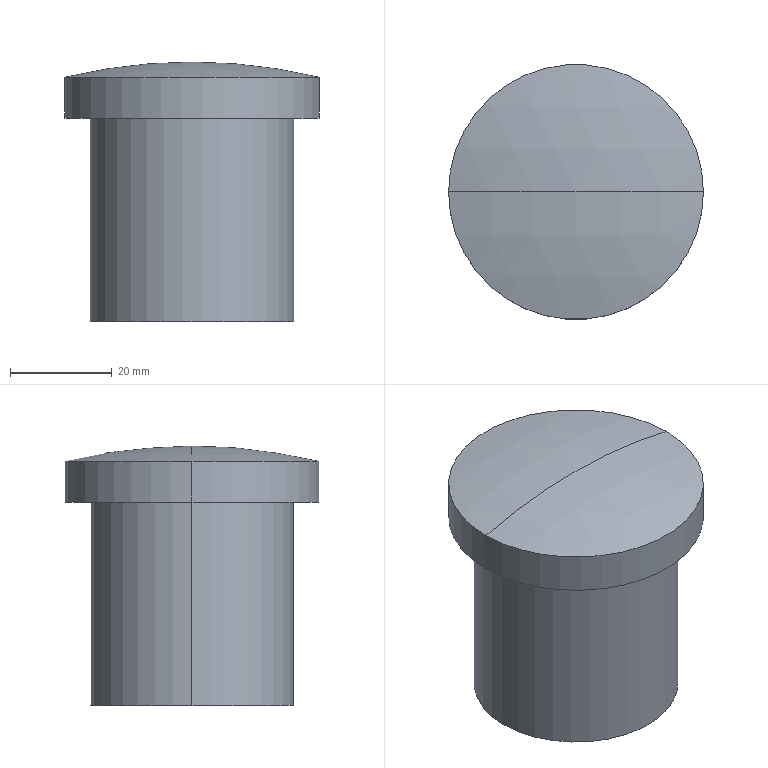Part | STEP file | Cylinder Joint | 1 solid | 11 faces | box 50 x 50 x 51 mm | volume 50075 mm3 | cylinder 6 | plane 3 | sphere 2 | commonest cylinder face diameters 24.5 x2 40 x2 50 x2
STEP:
#1=CARTESIAN_POINT('',(0.,0.,0.));
#2=DIRECTION('',(0.,0.,1.));
#3=DIRECTION('',(1.,0.,0.));
#4=AXIS2_PLACEMENT_3D('',#1,#2,#3);
#5=CARTESIAN_POINT('',(-12.25,0.,40.));
#6=VERTEX_POINT('',#5);
#7=CARTESIAN_POINT('',(-12.25,0.,0.));
#8=VERTEX_POINT('',#7);
#9=CARTESIAN_POINT('',(-12.25,0.,40.));
#10=DIRECTION('',(0.,0.,-1.));
#11=VECTOR('',#10,1.);
#12=LINE('',#9,#11);
#13=CARTESIAN_POINT('',(0.,0.,40.));
#14=DIRECTION('',(0.,0.,-1.));
#15=DIRECTION('',(-1.,0.,0.));
#16=AXIS2_PLACEMENT_3D('',#13,#14,#15);
#17=CYLINDRICAL_SURFACE('',#16,12.25);
#18=CARTESIAN_POINT('',(6.283,0.));
#19=DIRECTION('',(0.,1.));
#20=VECTOR('',#19,1.);
#21=LINE('',#18,#20);
#22=(GEOMETRIC_REPRESENTATION_CONTEXT(2)PARAMETRIC_REPRESENTATION_CONTEXT()REPRESENTATION_CONTEXT('',''));
#23=DEFINITIONAL_REPRESENTATION('',(#21),#22);
#24=PCURVE('',#17,#23);
#25=CARTESIAN_POINT('',(0.,0.,40.));
#26=DIRECTION('',(0.,0.,-1.));
#27=DIRECTION('',(-1.,0.,0.));
#28=AXIS2_PLACEMENT_3D('',#25,#26,#27);
#29=CYLINDRICAL_SURFACE('',#28,12.25);
#30=CARTESIAN_POINT('',(0.,0.));
#31=DIRECTION('',(0.,1.));
#32=VECTOR('',#31,1.);
#33=LINE('',#30,#32);
#34=(GEOMETRIC_REPRESENTATION_CONTEXT(2)PARAMETRIC_REPRESENTATION_CONTEXT()REPRESENTATION_CONTEXT('',''));
#35=DEFINITIONAL_REPRESENTATION('',(#33),#34);
#36=PCURVE('',#29,#35);
#37=SURFACE_CURVE('',#12,(#24,#36),.PCURVE_S1.);
#38=EDGE_CURVE('',#6,#8,#37,.T.);
#39=ORIENTED_EDGE('',*,*,#38,.T.);
#40=CARTESIAN_POINT('',(12.25,0.,0.));
#41=VERTEX_POINT('',#40);
#42=CARTESIAN_POINT('',(0.,0.,0.));
#43=DIRECTION('',(0.,0.,-1.));
#44=DIRECTION('',(-1.,0.,0.));
#45=AXIS2_PLACEMENT_3D('',#42,#43,#44);
#46=CIRCLE('',#45,12.25);
#47=CARTESIAN_POINT('',(0.,40.));
#48=DIRECTION('',(1.,0.));
#49=VECTOR('',#48,1.);
#50=LINE('',#47,#49);
#51=(GEOMETRIC_REPRESENTATION_CONTEXT(2)PARAMETRIC_REPRESENTATION_CONTEXT()REPRESENTATION_CONTEXT('',''));
#52=DEFINITIONAL_REPRESENTATION('',(#50),#51);
#53=PCURVE('',#17,#52);
#54=CARTESIAN_POINT('',(0.,0.,0.));
#55=DIRECTION('',(0.,0.,1.));
#56=DIRECTION('',(1.,0.,0.));
#57=AXIS2_PLACEMENT_3D('',#54,#55,#56);
#58=PLANE('',#57);
#59=CARTESIAN_POINT('',(-12.25,0.));
#60=CARTESIAN_POINT('',(-12.25,21.218));
#61=CARTESIAN_POINT('',(6.125,10.609));
#62=CARTESIAN_POINT('',(24.5,0.));
#63=CARTESIAN_POINT('',(6.125,-10.609));
#64=CARTESIAN_POINT('',(-12.25,-21.218));
#65=CARTESIAN_POINT('',(-12.25,0.));
#66=(BOUNDED_CURVE()B_SPLINE_CURVE(2,(#59,#60,#61,#62,#63,#64,#65),.UNSPECIFIED.,.T.,.F.)B_SPLINE_CURVE_WITH_KNOTS((1,2,2,2,2,1),(-2.094,0.,2.094,4.189,6.283,8.378),.UNSPECIFIED.)CURVE()GEOMETRIC_REPRESENTATION_ITEM()RATIONAL_B_SPLINE_CURVE((1.,0.5,1.,0.5,1.,0.5,1.))REPRESENTATION_ITEM(''));
#67=(GEOMETRIC_REPRESENTATION_CONTEXT(2)PARAMETRIC_REPRESENTATION_CONTEXT()REPRESENTATION_CONTEXT('',''));
#68=DEFINITIONAL_REPRESENTATION('',(#66),#67);
#69=PCURVE('',#58,#68);
#70=SURFACE_CURVE('',#46,(#53,#69),.PCURVE_S1.);
#71=EDGE_CURVE('',#41,#8,#70,.T.);
#72=ORIENTED_EDGE('',*,*,#71,.F.);
#73=CARTESIAN_POINT('',(12.25,0.,40.));
#74=VERTEX_POINT('',#73);
#75=CARTESIAN_POINT('',(12.25,0.,40.));
#76=DIRECTION('',(0.,0.,-1.));
#77=VECTOR('',#76,1.);
#78=LINE('',#75,#77);
#79=CARTESIAN_POINT('',(3.142,0.));
#80=DIRECTION('',(0.,1.));
#81=VECTOR('',#80,1.);
#82=LINE('',#79,#81);
#83=(GEOMETRIC_REPRESENTATION_CONTEXT(2)PARAMETRIC_REPRESENTATION_CONTEXT()REPRESENTATION_CONTEXT('',''));
#84=DEFINITIONAL_REPRESENTATION('',(#82),#83);
#85=PCURVE('',#17,#84);
#86=CARTESIAN_POINT('',(3.142,0.));
#87=DIRECTION('',(0.,1.));
#88=VECTOR('',#87,1.);
#89=LINE('',#86,#88);
#90=(GEOMETRIC_REPRESENTATION_CONTEXT(2)PARAMETRIC_REPRESENTATION_CONTEXT()REPRESENTATION_CONTEXT('',''));
#91=DEFINITIONAL_REPRESENTATION('',(#89),#90);
#92=PCURVE('',#29,#91);
#93=SURFACE_CURVE('',#78,(#85,#92),.PCURVE_S1.);
#94=EDGE_CURVE('',#74,#41,#93,.T.);
#95=ORIENTED_EDGE('',*,*,#94,.F.);
#96=CARTESIAN_POINT('',(0.,0.,40.));
#97=DIRECTION('',(0.,0.,-1.));
#98=DIRECTION('',(-1.,0.,0.));
#99=AXIS2_PLACEMENT_3D('',#96,#97,#98);
#100=CIRCLE('',#99,12.25);
#101=CARTESIAN_POINT('',(0.,0.));
#102=DIRECTION('',(1.,0.));
#103=VECTOR('',#102,1.);
#104=LINE('',#101,#103);
#105=(GEOMETRIC_REPRESENTATION_CONTEXT(2)PARAMETRIC_REPRESENTATION_CONTEXT()REPRESENTATION_CONTEXT('',''));
#106=DEFINITIONAL_REPRESENTATION('',(#104),#105);
#107=PCURVE('',#17,#106);
#108=CARTESIAN_POINT('',(0.,0.,40.));
#109=DIRECTION('',(0.,0.,-1.));
#110=DIRECTION('',(-1.,0.,0.));
#111=AXIS2_PLACEMENT_3D('',#108,#109,#110);
#112=PLANE('',#111);
#113=CARTESIAN_POINT('',(0.,0.));
#114=DIRECTION('',(1.,0.));
#115=AXIS2_PLACEMENT_2D('',#113,#114);
#116=CIRCLE('',#115,12.25);
#117=(GEOMETRIC_REPRESENTATION_CONTEXT(2)PARAMETRIC_REPRESENTATION_CONTEXT()REPRESENTATION_CONTEXT('',''));
#118=DEFINITIONAL_REPRESENTATION('',(#116),#117);
#119=PCURVE('',#112,#118);
#120=SURFACE_CURVE('',#100,(#107,#119),.PCURVE_S1.);
#121=EDGE_CURVE('',#74,#6,#120,.T.);
#122=ORIENTED_EDGE('',*,*,#121,.T.);
#123=EDGE_LOOP('',(#39,#72,#95,#122));
#124=FACE_BOUND('',#123,.F.);
#125=ADVANCED_FACE('',(#124),#17,.F.);
#126=CARTESIAN_POINT('',(25.,0.,48.));
#127=VERTEX_POINT('',#126);
#128=CARTESIAN_POINT('',(-25.,0.,48.));
#129=VERTEX_POINT('',#128);
#130=CARTESIAN_POINT('',(0.,0.,48.));
#131=DIRECTION('',(0.,0.,1.));
#132=DIRECTION('',(1.,0.,0.));
#133=AXIS2_PLACEMENT_3D('',#130,#131,#132);
#134=CIRCLE('',#133,25.);
#135=CARTESIAN_POINT('',(0.,0.,-54.667));
#136=DIRECTION('',(0.,1.,0.));
#137=DIRECTION('',(1.,0.,0.));
#138=AXIS2_PLACEMENT_3D('',#135,#136,#137);
#139=SPHERICAL_SURFACE('',#138,105.667);
#140=CARTESIAN_POINT('',(4.951,0.));
#141=CARTESIAN_POINT('',(4.951,0.01126));
#142=CARTESIAN_POINT('',(4.95,0.03379));
#143=CARTESIAN_POINT('',(4.943,0.06692));
#144=CARTESIAN_POINT('',(4.931,0.09876));
#145=CARTESIAN_POINT('',(4.915,0.1287));
#146=CARTESIAN_POINT('',(4.895,0.1561));
#147=CARTESIAN_POINT('',(4.871,0.1804));
#148=CARTESIAN_POINT('',(4.844,0.2011));
#149=CARTESIAN_POINT('',(4.814,0.2177));
#150=CARTESIAN_POINT('',(4.781,0.2298));
#151=CARTESIAN_POINT('',(4.747,0.2372));
#152=CARTESIAN_POINT('',(4.712,0.2397));
#153=CARTESIAN_POINT('',(4.678,0.2372));
#154=CARTESIAN_POINT('',(4.644,0.2298));
#155=CARTESIAN_POINT('',(4.611,0.2177));
#156=CARTESIAN_POINT('',(4.581,0.2011));
#157=CARTESIAN_POINT('',(4.554,0.1804));
#158=CARTESIAN_POINT('',(4.53,0.1561));
#159=CARTESIAN_POINT('',(4.51,0.1287));
#160=CARTESIAN_POINT('',(4.494,0.09876));
#161=CARTESIAN_POINT('',(4.482,0.06692));
#162=CARTESIAN_POINT('',(4.475,0.03379));
#163=CARTESIAN_POINT('',(4.474,0.01126));
#164=CARTESIAN_POINT('',(4.474,0.));
#165=B_SPLINE_CURVE_WITH_KNOTS('',3,(#140,#141,#142,#143,#144,#145,#146,#147,#148,#149,#150,#151,#152,#153,#154,#155,#156,#157,#158,#159,#160,#161,#162,#163,#164),.UNSPECIFIED.,.F.,.F.,(4,1,1,1,1,1,1,1,1,1,1,1,1,1,1,1,1,1,1,1,1,1,4),(0.,0.1428,0.2856,0.4284,0.5712,0.714,0.8568,0.9996,1.142,1.285,1.428,1.571,1.714,1.856,1.999,2.142,2.285,2.428,2.57,2.713,2.856,2.999,3.142),.QUASI_UNIFORM_KNOTS.);
#166=(GEOMETRIC_REPRESENTATION_CONTEXT(2)PARAMETRIC_REPRESENTATION_CONTEXT()REPRESENTATION_CONTEXT('',''));
#167=DEFINITIONAL_REPRESENTATION('',(#165),#166);
#168=PCURVE('',#139,#167);
#169=CARTESIAN_POINT('',(0.,0.,48.));
#170=DIRECTION('',(0.,0.,-1.));
#171=DIRECTION('',(-1.,0.,0.));
#172=AXIS2_PLACEMENT_3D('',#169,#170,#171);
#173=CYLINDRICAL_SURFACE('',#172,25.);
#174=CARTESIAN_POINT('',(3.142,0.));
#175=DIRECTION('',(-1.,0.));
#176=VECTOR('',#175,1.);
#177=LINE('',#174,#176);
#178=(GEOMETRIC_REPRESENTATION_CONTEXT(2)PARAMETRIC_REPRESENTATION_CONTEXT()REPRESENTATION_CONTEXT('',''));
#179=DEFINITIONAL_REPRESENTATION('',(#177),#178);
#180=PCURVE('',#173,#179);
#181=SURFACE_CURVE('',#134,(#168,#180),.PCURVE_S1.);
#182=EDGE_CURVE('',#127,#129,#181,.T.);
#183=ORIENTED_EDGE('',*,*,#182,.T.);
#184=CARTESIAN_POINT('',(0.,0.,51.));
#185=VERTEX_POINT('',#184);
#186=CARTESIAN_POINT('',(0.,0.,-54.667));
#187=DIRECTION('',(0.,1.,0.));
#188=DIRECTION('',(-1.,0.,0.));
#189=AXIS2_PLACEMENT_3D('',#186,#187,#188);
#190=CIRCLE('',#189,105.667);
#191=CARTESIAN_POINT('',(3.142,0.));
#192=DIRECTION('',(1.,0.));
#193=VECTOR('',#192,1.);
#194=LINE('',#191,#193);
#195=(GEOMETRIC_REPRESENTATION_CONTEXT(2)PARAMETRIC_REPRESENTATION_CONTEXT()REPRESENTATION_CONTEXT('',''));
#196=DEFINITIONAL_REPRESENTATION('',(#194),#195);
#197=PCURVE('',#139,#196);
#198=CARTESIAN_POINT('',(0.,0.,-54.667));
#199=DIRECTION('',(0.,1.,0.));
#200=DIRECTION('',(1.,0.,0.));
#201=AXIS2_PLACEMENT_3D('',#198,#199,#200);
#202=SPHERICAL_SURFACE('',#201,105.667);
#203=CARTESIAN_POINT('',(3.142,0.));
#204=DIRECTION('',(1.,0.));
#205=VECTOR('',#204,1.);
#206=LINE('',#203,#205);
#207=(GEOMETRIC_REPRESENTATION_CONTEXT(2)PARAMETRIC_REPRESENTATION_CONTEXT()REPRESENTATION_CONTEXT('',''));
#208=DEFINITIONAL_REPRESENTATION('',(#206),#207);
#209=PCURVE('',#202,#208);
#210=SURFACE_CURVE('',#190,(#197,#209),.PCURVE_S1.);
#211=EDGE_CURVE('',#129,#185,#210,.T.);
#212=ORIENTED_EDGE('',*,*,#211,.T.);
#213=CARTESIAN_POINT('',(0.,0.,-54.667));
#214=DIRECTION('',(0.,-1.,0.));
#215=DIRECTION('',(0.,0.,-1.));
#216=AXIS2_PLACEMENT_3D('',#213,#214,#215);
#217=CIRCLE('',#216,105.667);
#218=CARTESIAN_POINT('',(7.854,0.));
#219=DIRECTION('',(-1.,0.));
#220=VECTOR('',#219,1.);
#221=LINE('',#218,#220);
#222=(GEOMETRIC_REPRESENTATION_CONTEXT(2)PARAMETRIC_REPRESENTATION_CONTEXT()REPRESENTATION_CONTEXT('',''));
#223=DEFINITIONAL_REPRESENTATION('',(#221),#222);
#224=PCURVE('',#139,#223);
#225=CARTESIAN_POINT('',(7.854,0.));
#226=DIRECTION('',(-1.,0.));
#227=VECTOR('',#226,1.);
#228=LINE('',#225,#227);
#229=(GEOMETRIC_REPRESENTATION_CONTEXT(2)PARAMETRIC_REPRESENTATION_CONTEXT()REPRESENTATION_CONTEXT('',''));
#230=DEFINITIONAL_REPRESENTATION('',(#228),#229);
#231=PCURVE('',#202,#230);
#232=SURFACE_CURVE('',#217,(#224,#231),.PCURVE_S1.);
#233=EDGE_CURVE('',#127,#185,#232,.T.);
#234=ORIENTED_EDGE('',*,*,#233,.F.);
#235=EDGE_LOOP('',(#183,#212,#234));
#236=FACE_BOUND('',#235,.T.);
#237=ADVANCED_FACE('',(#236),#139,.T.);
#238=ORIENTED_EDGE('',*,*,#182,.F.);
#239=CARTESIAN_POINT('',(25.,0.,40.));
#240=VERTEX_POINT('',#239);
#241=CARTESIAN_POINT('',(25.,0.,48.));
#242=DIRECTION('',(0.,0.,-1.));
#243=VECTOR('',#242,1.);
#244=LINE('',#241,#243);
#245=CARTESIAN_POINT('',(3.142,0.));
#246=DIRECTION('',(0.,1.));
#247=VECTOR('',#246,1.);
#248=LINE('',#245,#247);
#249=(GEOMETRIC_REPRESENTATION_CONTEXT(2)PARAMETRIC_REPRESENTATION_CONTEXT()REPRESENTATION_CONTEXT('',''));
#250=DEFINITIONAL_REPRESENTATION('',(#248),#249);
#251=PCURVE('',#173,#250);
#252=CARTESIAN_POINT('',(0.,0.,48.));
#253=DIRECTION('',(0.,0.,-1.));
#254=DIRECTION('',(-1.,0.,0.));
#255=AXIS2_PLACEMENT_3D('',#252,#253,#254);
#256=CYLINDRICAL_SURFACE('',#255,25.);
#257=CARTESIAN_POINT('',(3.142,0.));
#258=DIRECTION('',(0.,1.));
#259=VECTOR('',#258,1.);
#260=LINE('',#257,#259);
#261=(GEOMETRIC_REPRESENTATION_CONTEXT(2)PARAMETRIC_REPRESENTATION_CONTEXT()REPRESENTATION_CONTEXT('',''));
#262=DEFINITIONAL_REPRESENTATION('',(#260),#261);
#263=PCURVE('',#256,#262);
#264=SURFACE_CURVE('',#244,(#251,#263),.PCURVE_S1.);
#265=EDGE_CURVE('',#127,#240,#264,.T.);
#266=ORIENTED_EDGE('',*,*,#265,.T.);
#267=CARTESIAN_POINT('',(-25.,0.,40.));
#268=VERTEX_POINT('',#267);
#269=CARTESIAN_POINT('',(0.,0.,40.));
#270=DIRECTION('',(0.,0.,1.));
#271=DIRECTION('',(1.,0.,0.));
#272=AXIS2_PLACEMENT_3D('',#269,#270,#271);
#273=CIRCLE('',#272,25.);
#274=CARTESIAN_POINT('',(3.142,8.));
#275=DIRECTION('',(-1.,0.));
#276=VECTOR('',#275,1.);
#277=LINE('',#274,#276);
#278=(GEOMETRIC_REPRESENTATION_CONTEXT(2)PARAMETRIC_REPRESENTATION_CONTEXT()REPRESENTATION_CONTEXT('',''));
#279=DEFINITIONAL_REPRESENTATION('',(#277),#278);
#280=PCURVE('',#173,#279);
#281=CARTESIAN_POINT('',(0.,0.,40.));
#282=DIRECTION('',(0.,0.,1.));
#283=DIRECTION('',(1.,0.,0.));
#284=AXIS2_PLACEMENT_3D('',#281,#282,#283);
#285=PLANE('',#284);
#286=CARTESIAN_POINT('',(0.,0.));
#287=DIRECTION('',(1.,0.));
#288=AXIS2_PLACEMENT_2D('',#286,#287);
#289=CIRCLE('',#288,25.);
#290=(GEOMETRIC_REPRESENTATION_CONTEXT(2)PARAMETRIC_REPRESENTATION_CONTEXT()REPRESENTATION_CONTEXT('',''));
#291=DEFINITIONAL_REPRESENTATION('',(#289),#290);
#292=PCURVE('',#285,#291);
#293=SURFACE_CURVE('',#273,(#280,#292),.PCURVE_S1.);
#294=EDGE_CURVE('',#240,#268,#293,.T.);
#295=ORIENTED_EDGE('',*,*,#294,.T.);
#296=CARTESIAN_POINT('',(-25.,0.,48.));
#297=DIRECTION('',(0.,0.,-1.));
#298=VECTOR('',#297,1.);
#299=LINE('',#296,#298);
#300=CARTESIAN_POINT('',(0.,0.));
#301=DIRECTION('',(0.,1.));
#302=VECTOR('',#301,1.);
#303=LINE('',#300,#302);
#304=(GEOMETRIC_REPRESENTATION_CONTEXT(2)PARAMETRIC_REPRESENTATION_CONTEXT()REPRESENTATION_CONTEXT('',''));
#305=DEFINITIONAL_REPRESENTATION('',(#303),#304);
#306=PCURVE('',#173,#305);
#307=CARTESIAN_POINT('',(6.283,0.));
#308=DIRECTION('',(0.,1.));
#309=VECTOR('',#308,1.);
#310=LINE('',#307,#309);
#311=(GEOMETRIC_REPRESENTATION_CONTEXT(2)PARAMETRIC_REPRESENTATION_CONTEXT()REPRESENTATION_CONTEXT('',''));
#312=DEFINITIONAL_REPRESENTATION('',(#310),#311);
#313=PCURVE('',#256,#312);
#314=SURFACE_CURVE('',#299,(#306,#313),.PCURVE_S1.);
#315=EDGE_CURVE('',#129,#268,#314,.T.);
#316=ORIENTED_EDGE('',*,*,#315,.F.);
#317=EDGE_LOOP('',(#238,#266,#295,#316));
#318=FACE_BOUND('',#317,.T.);
#319=ADVANCED_FACE('',(#318),#173,.T.);
#320=CARTESIAN_POINT('',(20.,0.,40.));
#321=VERTEX_POINT('',#320);
#322=CARTESIAN_POINT('',(-20.,0.,40.));
#323=VERTEX_POINT('',#322);
#324=CARTESIAN_POINT('',(0.,0.,40.));
#325=DIRECTION('',(0.,0.,1.));
#326=DIRECTION('',(1.,0.,0.));
#327=AXIS2_PLACEMENT_3D('',#324,#325,#326);
#328=CIRCLE('',#327,20.);
#329=CARTESIAN_POINT('',(0.,0.,40.));
#330=DIRECTION('',(0.,0.,-1.));
#331=DIRECTION('',(-1.,0.,0.));
#332=AXIS2_PLACEMENT_3D('',#329,#330,#331);
#333=CYLINDRICAL_SURFACE('',#332,20.);
#334=CARTESIAN_POINT('',(3.142,0.));
#335=DIRECTION('',(-1.,0.));
#336=VECTOR('',#335,1.);
#337=LINE('',#334,#336);
#338=(GEOMETRIC_REPRESENTATION_CONTEXT(2)PARAMETRIC_REPRESENTATION_CONTEXT()REPRESENTATION_CONTEXT('',''));
#339=DEFINITIONAL_REPRESENTATION('',(#337),#338);
#340=PCURVE('',#333,#339);
#341=CARTESIAN_POINT('',(0.,0.));
#342=DIRECTION('',(1.,0.));
#343=AXIS2_PLACEMENT_2D('',#341,#342);
#344=CIRCLE('',#343,20.);
#345=(GEOMETRIC_REPRESENTATION_CONTEXT(2)PARAMETRIC_REPRESENTATION_CONTEXT()REPRESENTATION_CONTEXT('',''));
#346=DEFINITIONAL_REPRESENTATION('',(#344),#345);
#347=PCURVE('',#285,#346);
#348=SURFACE_CURVE('',#328,(#340,#347),.PCURVE_S1.);
#349=EDGE_CURVE('',#321,#323,#348,.T.);
#350=ORIENTED_EDGE('',*,*,#349,.F.);
#351=CARTESIAN_POINT('',(20.,0.,0.));
#352=VERTEX_POINT('',#351);
#353=CARTESIAN_POINT('',(20.,0.,40.));
#354=DIRECTION('',(0.,0.,-1.));
#355=VECTOR('',#354,1.);
#356=LINE('',#353,#355);
#357=CARTESIAN_POINT('',(3.142,0.));
#358=DIRECTION('',(0.,1.));
#359=VECTOR('',#358,1.);
#360=LINE('',#357,#359);
#361=(GEOMETRIC_REPRESENTATION_CONTEXT(2)PARAMETRIC_REPRESENTATION_CONTEXT()REPRESENTATION_CONTEXT('',''));
#362=DEFINITIONAL_REPRESENTATION('',(#360),#361);
#363=PCURVE('',#333,#362);
#364=CARTESIAN_POINT('',(0.,0.,40.));
#365=DIRECTION('',(0.,0.,-1.));
#366=DIRECTION('',(-1.,0.,0.));
#367=AXIS2_PLACEMENT_3D('',#364,#365,#366);
#368=CYLINDRICAL_SURFACE('',#367,20.);
#369=CARTESIAN_POINT('',(3.142,0.));
#370=DIRECTION('',(0.,1.));
#371=VECTOR('',#370,1.);
#372=LINE('',#369,#371);
#373=(GEOMETRIC_REPRESENTATION_CONTEXT(2)PARAMETRIC_REPRESENTATION_CONTEXT()REPRESENTATION_CONTEXT('',''));
#374=DEFINITIONAL_REPRESENTATION('',(#372),#373);
#375=PCURVE('',#368,#374);
#376=SURFACE_CURVE('',#356,(#363,#375),.PCURVE_S1.);
#377=EDGE_CURVE('',#321,#352,#376,.T.);
#378=ORIENTED_EDGE('',*,*,#377,.T.);
#379=CARTESIAN_POINT('',(-20.,0.,0.));
#380=VERTEX_POINT('',#379);
#381=CARTESIAN_POINT('',(0.,0.,0.));
#382=DIRECTION('',(0.,0.,1.));
#383=DIRECTION('',(1.,0.,0.));
#384=AXIS2_PLACEMENT_3D('',#381,#382,#383);
#385=CIRCLE('',#384,20.);
#386=CARTESIAN_POINT('',(3.142,40.));
#387=DIRECTION('',(-1.,0.));
#388=VECTOR('',#387,1.);
#389=LINE('',#386,#388);
#390=(GEOMETRIC_REPRESENTATION_CONTEXT(2)PARAMETRIC_REPRESENTATION_CONTEXT()REPRESENTATION_CONTEXT('',''));
#391=DEFINITIONAL_REPRESENTATION('',(#389),#390);
#392=PCURVE('',#333,#391);
#393=CARTESIAN_POINT('',(0.,0.));
#394=DIRECTION('',(1.,0.));
#395=AXIS2_PLACEMENT_2D('',#393,#394);
#396=CIRCLE('',#395,20.);
#397=(GEOMETRIC_REPRESENTATION_CONTEXT(2)PARAMETRIC_REPRESENTATION_CONTEXT()REPRESENTATION_CONTEXT('',''));
#398=DEFINITIONAL_REPRESENTATION('',(#396),#397);
#399=PCURVE('',#58,#398);
#400=SURFACE_CURVE('',#385,(#392,#399),.PCURVE_S1.);
#401=EDGE_CURVE('',#352,#380,#400,.T.);
#402=ORIENTED_EDGE('',*,*,#401,.T.);
#403=CARTESIAN_POINT('',(-20.,0.,40.));
#404=DIRECTION('',(0.,0.,-1.));
#405=VECTOR('',#404,1.);
#406=LINE('',#403,#405);
#407=CARTESIAN_POINT('',(0.,0.));
#408=DIRECTION('',(0.,1.));
#409=VECTOR('',#408,1.);
#410=LINE('',#407,#409);
#411=(GEOMETRIC_REPRESENTATION_CONTEXT(2)PARAMETRIC_REPRESENTATION_CONTEXT()REPRESENTATION_CONTEXT('',''));
#412=DEFINITIONAL_REPRESENTATION('',(#410),#411);
#413=PCURVE('',#333,#412);
#414=CARTESIAN_POINT('',(6.283,0.));
#415=DIRECTION('',(0.,1.));
#416=VECTOR('',#415,1.);
#417=LINE('',#414,#416);
#418=(GEOMETRIC_REPRESENTATION_CONTEXT(2)PARAMETRIC_REPRESENTATION_CONTEXT()REPRESENTATION_CONTEXT('',''));
#419=DEFINITIONAL_REPRESENTATION('',(#417),#418);
#420=PCURVE('',#368,#419);
#421=SURFACE_CURVE('',#406,(#413,#420),.PCURVE_S1.);
#422=EDGE_CURVE('',#323,#380,#421,.T.);
#423=ORIENTED_EDGE('',*,*,#422,.F.);
#424=EDGE_LOOP('',(#350,#378,#402,#423));
#425=FACE_BOUND('',#424,.T.);
#426=ADVANCED_FACE('',(#425),#333,.T.);
#427=ORIENTED_EDGE('',*,*,#377,.F.);
#428=CARTESIAN_POINT('',(0.,0.,40.));
#429=DIRECTION('',(0.,0.,1.));
#430=DIRECTION('',(1.,0.,0.));
#431=AXIS2_PLACEMENT_3D('',#428,#429,#430);
#432=CIRCLE('',#431,20.);
#433=CARTESIAN_POINT('',(9.425,0.));
#434=DIRECTION('',(-1.,0.));
#435=VECTOR('',#434,1.);
#436=LINE('',#433,#435);
#437=(GEOMETRIC_REPRESENTATION_CONTEXT(2)PARAMETRIC_REPRESENTATION_CONTEXT()REPRESENTATION_CONTEXT('',''));
#438=DEFINITIONAL_REPRESENTATION('',(#436),#437);
#439=PCURVE('',#368,#438);
#440=CARTESIAN_POINT('',(0.,0.));
#441=DIRECTION('',(1.,0.));
#442=AXIS2_PLACEMENT_2D('',#440,#441);
#443=CIRCLE('',#442,20.);
#444=(GEOMETRIC_REPRESENTATION_CONTEXT(2)PARAMETRIC_REPRESENTATION_CONTEXT()REPRESENTATION_CONTEXT('',''));
#445=DEFINITIONAL_REPRESENTATION('',(#443),#444);
#446=PCURVE('',#285,#445);
#447=SURFACE_CURVE('',#432,(#439,#446),.PCURVE_S1.);
#448=EDGE_CURVE('',#323,#321,#447,.T.);
#449=ORIENTED_EDGE('',*,*,#448,.F.);
#450=ORIENTED_EDGE('',*,*,#422,.T.);
#451=CARTESIAN_POINT('',(0.,0.,0.));
#452=DIRECTION('',(0.,0.,1.));
#453=DIRECTION('',(1.,0.,0.));
#454=AXIS2_PLACEMENT_3D('',#451,#452,#453);
#455=CIRCLE('',#454,20.);
#456=CARTESIAN_POINT('',(9.425,40.));
#457=DIRECTION('',(-1.,0.));
#458=VECTOR('',#457,1.);
#459=LINE('',#456,#458);
#460=(GEOMETRIC_REPRESENTATION_CONTEXT(2)PARAMETRIC_REPRESENTATION_CONTEXT()REPRESENTATION_CONTEXT('',''));
#461=DEFINITIONAL_REPRESENTATION('',(#459),#460);
#462=PCURVE('',#368,#461);
#463=CARTESIAN_POINT('',(0.,0.));
#464=DIRECTION('',(1.,0.));
#465=AXIS2_PLACEMENT_2D('',#463,#464);
#466=CIRCLE('',#465,20.);
#467=(GEOMETRIC_REPRESENTATION_CONTEXT(2)PARAMETRIC_REPRESENTATION_CONTEXT()REPRESENTATION_CONTEXT('',''));
#468=DEFINITIONAL_REPRESENTATION('',(#466),#467);
#469=PCURVE('',#58,#468);
#470=SURFACE_CURVE('',#455,(#462,#469),.PCURVE_S1.);
#471=EDGE_CURVE('',#380,#352,#470,.T.);
#472=ORIENTED_EDGE('',*,*,#471,.T.);
#473=EDGE_LOOP('',(#427,#449,#450,#472));
#474=FACE_BOUND('',#473,.T.);
#475=ADVANCED_FACE('',(#474),#368,.T.);
#476=CARTESIAN_POINT('',(0.,0.,0.));
#477=DIRECTION('',(0.,0.,-1.));
#478=DIRECTION('',(-1.,0.,0.));
#479=AXIS2_PLACEMENT_3D('',#476,#477,#478);
#480=CIRCLE('',#479,12.25);
#481=CARTESIAN_POINT('',(-12.25,0.));
#482=CARTESIAN_POINT('',(-12.25,21.218));
#483=CARTESIAN_POINT('',(6.125,10.609));
#484=CARTESIAN_POINT('',(24.5,0.));
#485=CARTESIAN_POINT('',(6.125,-10.609));
#486=CARTESIAN_POINT('',(-12.25,-21.218));
#487=CARTESIAN_POINT('',(-12.25,0.));
#488=(BOUNDED_CURVE()B_SPLINE_CURVE(2,(#481,#482,#483,#484,#485,#486,#487),.UNSPECIFIED.,.T.,.F.)B_SPLINE_CURVE_WITH_KNOTS((1,2,2,2,2,1),(-2.094,0.,2.094,4.189,6.283,8.378),.UNSPECIFIED.)CURVE()GEOMETRIC_REPRESENTATION_ITEM()RATIONAL_B_SPLINE_CURVE((1.,0.5,1.,0.5,1.,0.5,1.))REPRESENTATION_ITEM(''));
#489=(GEOMETRIC_REPRESENTATION_CONTEXT(2)PARAMETRIC_REPRESENTATION_CONTEXT()REPRESENTATION_CONTEXT('',''));
#490=DEFINITIONAL_REPRESENTATION('',(#488),#489);
#491=PCURVE('',#58,#490);
#492=CARTESIAN_POINT('',(0.,40.));
#493=DIRECTION('',(1.,0.));
#494=VECTOR('',#493,1.);
#495=LINE('',#492,#494);
#496=(GEOMETRIC_REPRESENTATION_CONTEXT(2)PARAMETRIC_REPRESENTATION_CONTEXT()REPRESENTATION_CONTEXT('',''));
#497=DEFINITIONAL_REPRESENTATION('',(#495),#496);
#498=PCURVE('',#29,#497);
#499=SURFACE_CURVE('',#480,(#491,#498),.PCURVE_S1.);
#500=EDGE_CURVE('',#8,#41,#499,.T.);
#501=ORIENTED_EDGE('',*,*,#500,.F.);
#502=ORIENTED_EDGE('',*,*,#71,.F.);
#503=EDGE_LOOP('',(#501,#502));
#504=FACE_BOUND('',#503,.T.);
#505=ORIENTED_EDGE('',*,*,#471,.F.);
#506=ORIENTED_EDGE('',*,*,#401,.F.);
#507=EDGE_LOOP('',(#505,#506));
#508=FACE_BOUND('',#507,.T.);
#509=ADVANCED_FACE('',(#504,#508),#58,.F.);
#510=CARTESIAN_POINT('',(0.,0.,40.));
#511=DIRECTION('',(0.,0.,1.));
#512=DIRECTION('',(1.,0.,0.));
#513=AXIS2_PLACEMENT_3D('',#510,#511,#512);
#514=CIRCLE('',#513,25.);
#515=CARTESIAN_POINT('',(0.,0.));
#516=DIRECTION('',(1.,0.));
#517=AXIS2_PLACEMENT_2D('',#515,#516);
#518=CIRCLE('',#517,25.);
#519=(GEOMETRIC_REPRESENTATION_CONTEXT(2)PARAMETRIC_REPRESENTATION_CONTEXT()REPRESENTATION_CONTEXT('',''));
#520=DEFINITIONAL_REPRESENTATION('',(#518),#519);
#521=PCURVE('',#285,#520);
#522=CARTESIAN_POINT('',(9.425,8.));
#523=DIRECTION('',(-1.,0.));
#524=VECTOR('',#523,1.);
#525=LINE('',#522,#524);
#526=(GEOMETRIC_REPRESENTATION_CONTEXT(2)PARAMETRIC_REPRESENTATION_CONTEXT()REPRESENTATION_CONTEXT('',''));
#527=DEFINITIONAL_REPRESENTATION('',(#525),#526);
#528=PCURVE('',#256,#527);
#529=SURFACE_CURVE('',#514,(#521,#528),.PCURVE_S1.);
#530=EDGE_CURVE('',#268,#240,#529,.T.);
#531=ORIENTED_EDGE('',*,*,#530,.F.);
#532=ORIENTED_EDGE('',*,*,#294,.F.);
#533=EDGE_LOOP('',(#531,#532));
#534=FACE_BOUND('',#533,.T.);
#535=ORIENTED_EDGE('',*,*,#448,.T.);
#536=ORIENTED_EDGE('',*,*,#349,.T.);
#537=EDGE_LOOP('',(#535,#536));
#538=FACE_BOUND('',#537,.T.);
#539=ADVANCED_FACE('',(#534,#538),#285,.F.);
#540=ORIENTED_EDGE('',*,*,#265,.F.);
#541=CARTESIAN_POINT('',(0.,0.,48.));
#542=DIRECTION('',(0.,0.,1.));
#543=DIRECTION('',(1.,0.,0.));
#544=AXIS2_PLACEMENT_3D('',#541,#542,#543);
#545=CIRCLE('',#544,25.);
#546=CARTESIAN_POINT('',(9.425,0.));
#547=DIRECTION('',(-1.,0.));
#548=VECTOR('',#547,1.);
#549=LINE('',#546,#548);
#550=(GEOMETRIC_REPRESENTATION_CONTEXT(2)PARAMETRIC_REPRESENTATION_CONTEXT()REPRESENTATION_CONTEXT('',''));
#551=DEFINITIONAL_REPRESENTATION('',(#549),#550);
#552=PCURVE('',#256,#551);
#553=CARTESIAN_POINT('',(4.474,0.));
#554=CARTESIAN_POINT('',(4.474,-0.01126));
#555=CARTESIAN_POINT('',(4.475,-0.03379));
#556=CARTESIAN_POINT('',(4.482,-0.06692));
#557=CARTESIAN_POINT('',(4.494,-0.09876));
#558=CARTESIAN_POINT('',(4.51,-0.1287));
#559=CARTESIAN_POINT('',(4.53,-0.1561));
#560=CARTESIAN_POINT('',(4.554,-0.1804));
#561=CARTESIAN_POINT('',(4.581,-0.2011));
#562=CARTESIAN_POINT('',(4.611,-0.2177));
#563=CARTESIAN_POINT('',(4.644,-0.2298));
#564=CARTESIAN_POINT('',(4.678,-0.2372));
#565=CARTESIAN_POINT('',(4.712,-0.2397));
#566=CARTESIAN_POINT('',(4.747,-0.2372));
#567=CARTESIAN_POINT('',(4.781,-0.2298));
#568=CARTESIAN_POINT('',(4.814,-0.2177));
#569=CARTESIAN_POINT('',(4.844,-0.2011));
#570=CARTESIAN_POINT('',(4.871,-0.1804));
#571=CARTESIAN_POINT('',(4.895,-0.1561));
#572=CARTESIAN_POINT('',(4.915,-0.1287));
#573=CARTESIAN_POINT('',(4.931,-0.09876));
#574=CARTESIAN_POINT('',(4.943,-0.06692));
#575=CARTESIAN_POINT('',(4.95,-0.03379));
#576=CARTESIAN_POINT('',(4.951,-0.01126));
#577=CARTESIAN_POINT('',(4.951,0.));
#578=B_SPLINE_CURVE_WITH_KNOTS('',3,(#553,#554,#555,#556,#557,#558,#559,#560,#561,#562,#563,#564,#565,#566,#567,#568,#569,#570,#571,#572,#573,#574,#575,#576,#577),.UNSPECIFIED.,.F.,.F.,(4,1,1,1,1,1,1,1,1,1,1,1,1,1,1,1,1,1,1,1,1,1,4),(3.142,3.284,3.427,3.57,3.713,3.856,3.998,4.141,4.284,4.427,4.57,4.712,4.855,4.998,5.141,5.284,5.426,5.569,5.712,5.855,5.998,6.14,6.283),.QUASI_UNIFORM_KNOTS.);
#579=(GEOMETRIC_REPRESENTATION_CONTEXT(2)PARAMETRIC_REPRESENTATION_CONTEXT()REPRESENTATION_CONTEXT('',''));
#580=DEFINITIONAL_REPRESENTATION('',(#578),#579);
#581=PCURVE('',#202,#580);
#582=SURFACE_CURVE('',#545,(#552,#581),.PCURVE_S1.);
#583=EDGE_CURVE('',#129,#127,#582,.T.);
#584=ORIENTED_EDGE('',*,*,#583,.F.);
#585=ORIENTED_EDGE('',*,*,#315,.T.);
#586=ORIENTED_EDGE('',*,*,#530,.T.);
#587=EDGE_LOOP('',(#540,#584,#585,#586));
#588=FACE_BOUND('',#587,.T.);
#589=ADVANCED_FACE('',(#588),#256,.T.);
#590=ORIENTED_EDGE('',*,*,#211,.F.);
#591=ORIENTED_EDGE('',*,*,#583,.T.);
#592=ORIENTED_EDGE('',*,*,#233,.T.);
#593=EDGE_LOOP('',(#590,#591,#592));
#594=FACE_BOUND('',#593,.T.);
#595=ADVANCED_FACE('',(#594),#202,.T.);
#596=ORIENTED_EDGE('',*,*,#500,.F.);
#597=ORIENTED_EDGE('',*,*,#38,.F.);
#598=CARTESIAN_POINT('',(0.,0.,40.));
#599=DIRECTION('',(0.,0.,-1.));
#600=DIRECTION('',(-1.,0.,0.));
#601=AXIS2_PLACEMENT_3D('',#598,#599,#600);
#602=CIRCLE('',#601,12.25);
#603=CARTESIAN_POINT('',(0.,0.));
#604=DIRECTION('',(1.,0.));
#605=VECTOR('',#604,1.);
#606=LINE('',#603,#605);
#607=(GEOMETRIC_REPRESENTATION_CONTEXT(2)PARAMETRIC_REPRESENTATION_CONTEXT()REPRESENTATION_CONTEXT('',''));
#608=DEFINITIONAL_REPRESENTATION('',(#606),#607);
#609=PCURVE('',#29,#608);
#610=CARTESIAN_POINT('',(0.,0.));
#611=DIRECTION('',(1.,0.));
#612=AXIS2_PLACEMENT_2D('',#610,#611);
#613=CIRCLE('',#612,12.25);
#614=(GEOMETRIC_REPRESENTATION_CONTEXT(2)PARAMETRIC_REPRESENTATION_CONTEXT()REPRESENTATION_CONTEXT('',''));
#615=DEFINITIONAL_REPRESENTATION('',(#613),#614);
#616=PCURVE('',#112,#615);
#617=SURFACE_CURVE('',#602,(#609,#616),.PCURVE_S1.);
#618=EDGE_CURVE('',#6,#74,#617,.T.);
#619=ORIENTED_EDGE('',*,*,#618,.T.);
#620=ORIENTED_EDGE('',*,*,#94,.T.);
#621=EDGE_LOOP('',(#596,#597,#619,#620));
#622=FACE_BOUND('',#621,.F.);
#623=ADVANCED_FACE('',(#622),#29,.F.);
#624=ORIENTED_EDGE('',*,*,#618,.T.);
#625=ORIENTED_EDGE('',*,*,#121,.T.);
#626=EDGE_LOOP('',(#624,#625));
#627=FACE_BOUND('',#626,.T.);
#628=ADVANCED_FACE('',(#627),#112,.T.);
#629=CLOSED_SHELL('',(#125,#237,#319,#426,#475,#509,#539,#589,#595,#623,#628));
#630=MANIFOLD_SOLID_BREP('',#629);
#631=(LENGTH_UNIT()NAMED_UNIT(*)SI_UNIT(.MILLI.,.METRE.));
#632=UNCERTAINTY_MEASURE_WITH_UNIT(LENGTH_MEASURE(0.0000001),#631,'','');
#633=(NAMED_UNIT(*)PLANE_ANGLE_UNIT()SI_UNIT($,.RADIAN.));
#634=(NAMED_UNIT(*)SI_UNIT($,.STERADIAN.)SOLID_ANGLE_UNIT());
#635=(GEOMETRIC_REPRESENTATION_CONTEXT(3)GLOBAL_UNCERTAINTY_ASSIGNED_CONTEXT((#632))GLOBAL_UNIT_ASSIGNED_CONTEXT((#631,#633,#634))REPRESENTATION_CONTEXT('',''));
#636=ADVANCED_BREP_SHAPE_REPRESENTATION('',(#4,#630),#635);